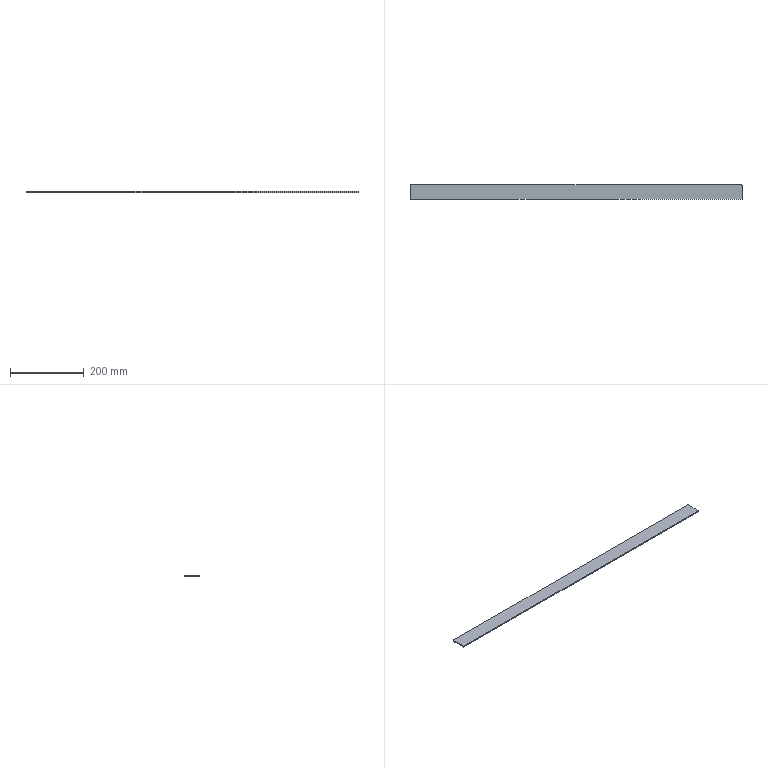Part | SolidWorks | features Extrusion 1, Fillet 1 | 1 solid | 8 faces | box 900 x 40 x 3 mm | volume 107995 mm3 | plane 6 | cylinder 2 | commonest cylinder face diameters 4 x2
STEP:
#1=CARTESIAN_POINT('',(450.,-20.,0.));
#2=VERTEX_POINT('',#1);
#3=CARTESIAN_POINT('',(450.,18.,0.));
#4=VERTEX_POINT('',#3);
#5=CARTESIAN_POINT('',(450.,20.,0.));
#6=DIRECTION('',(0.,1.,0.));
#7=VECTOR('',#6,1000.);
#8=LINE('',#5,#7);
#9=EDGE_CURVE('',#2,#4,#8,.T.);
#10=ORIENTED_EDGE('',*,*,#9,.T.);
#11=CARTESIAN_POINT('',(450.,18.,3.));
#12=VERTEX_POINT('',#11);
#13=CARTESIAN_POINT('',(450.,18.,3.));
#14=DIRECTION('',(0.,0.,1.));
#15=VECTOR('',#14,1000.);
#16=LINE('',#13,#15);
#17=EDGE_CURVE('',#4,#12,#16,.T.);
#18=ORIENTED_EDGE('',*,*,#17,.T.);
#19=CARTESIAN_POINT('',(450.,-20.,3.));
#20=VERTEX_POINT('',#19);
#21=CARTESIAN_POINT('',(450.,20.,3.));
#22=DIRECTION('',(0.,1.,0.));
#23=VECTOR('',#22,1000.);
#24=LINE('',#21,#23);
#25=EDGE_CURVE('',#20,#12,#24,.T.);
#26=ORIENTED_EDGE('',*,*,#25,.F.);
#27=CARTESIAN_POINT('',(450.,-20.,3.));
#28=DIRECTION('',(0.,0.,-1.));
#29=VECTOR('',#28,1000.);
#30=LINE('',#27,#29);
#31=EDGE_CURVE('',#20,#2,#30,.T.);
#32=ORIENTED_EDGE('',*,*,#31,.T.);
#33=EDGE_LOOP('',(#10,#18,#26,#32));
#34=FACE_OUTER_BOUND('',#33,.T.);
#35=CARTESIAN_POINT('',(450.,20.,3.));
#36=DIRECTION('',(-1.,0.,0.));
#37=DIRECTION('',(0.,0.,1.));
#38=AXIS2_PLACEMENT_3D('',#35,#36,#37);
#39=PLANE('',#38);
#40=ADVANCED_FACE('',(#34),#39,.F.);
#41=CARTESIAN_POINT('',(448.,20.,0.));
#42=VERTEX_POINT('',#41);
#43=CARTESIAN_POINT('',(-448.,20.,0.));
#44=VERTEX_POINT('',#43);
#45=CARTESIAN_POINT('',(-450.,20.,0.));
#46=DIRECTION('',(-1.,0.,0.));
#47=VECTOR('',#46,1000.);
#48=LINE('',#45,#47);
#49=EDGE_CURVE('',#42,#44,#48,.T.);
#50=ORIENTED_EDGE('',*,*,#49,.T.);
#51=CARTESIAN_POINT('',(-448.,20.,3.));
#52=VERTEX_POINT('',#51);
#53=CARTESIAN_POINT('',(-448.,20.,3.));
#54=DIRECTION('',(0.,0.,1.));
#55=VECTOR('',#54,1000.);
#56=LINE('',#53,#55);
#57=EDGE_CURVE('',#44,#52,#56,.T.);
#58=ORIENTED_EDGE('',*,*,#57,.T.);
#59=CARTESIAN_POINT('',(448.,20.,3.));
#60=VERTEX_POINT('',#59);
#61=CARTESIAN_POINT('',(-450.,20.,3.));
#62=DIRECTION('',(-1.,0.,0.));
#63=VECTOR('',#62,1000.);
#64=LINE('',#61,#63);
#65=EDGE_CURVE('',#60,#52,#64,.T.);
#66=ORIENTED_EDGE('',*,*,#65,.F.);
#67=CARTESIAN_POINT('',(448.,20.,3.));
#68=DIRECTION('',(0.,0.,-1.));
#69=VECTOR('',#68,1000.);
#70=LINE('',#67,#69);
#71=EDGE_CURVE('',#60,#42,#70,.T.);
#72=ORIENTED_EDGE('',*,*,#71,.T.);
#73=EDGE_LOOP('',(#50,#58,#66,#72));
#74=FACE_OUTER_BOUND('',#73,.T.);
#75=CARTESIAN_POINT('',(-450.,20.,3.));
#76=DIRECTION('',(0.,-1.,0.));
#77=DIRECTION('',(0.,0.,-1.));
#78=AXIS2_PLACEMENT_3D('',#75,#76,#77);
#79=PLANE('',#78);
#80=ADVANCED_FACE('',(#74),#79,.F.);
#81=CARTESIAN_POINT('',(-450.,18.,3.));
#82=VERTEX_POINT('',#81);
#83=CARTESIAN_POINT('',(-450.,-20.,3.));
#84=VERTEX_POINT('',#83);
#85=CARTESIAN_POINT('',(-450.,20.,3.));
#86=DIRECTION('',(0.,-1.,0.));
#87=VECTOR('',#86,1000.);
#88=LINE('',#85,#87);
#89=EDGE_CURVE('',#82,#84,#88,.T.);
#90=ORIENTED_EDGE('',*,*,#89,.F.);
#91=CARTESIAN_POINT('',(-450.,18.,0.));
#92=VERTEX_POINT('',#91);
#93=CARTESIAN_POINT('',(-450.,18.,3.));
#94=DIRECTION('',(0.,0.,-1.));
#95=VECTOR('',#94,1000.);
#96=LINE('',#93,#95);
#97=EDGE_CURVE('',#82,#92,#96,.T.);
#98=ORIENTED_EDGE('',*,*,#97,.T.);
#99=CARTESIAN_POINT('',(-450.,-20.,0.));
#100=VERTEX_POINT('',#99);
#101=CARTESIAN_POINT('',(-450.,20.,0.));
#102=DIRECTION('',(0.,-1.,0.));
#103=VECTOR('',#102,1000.);
#104=LINE('',#101,#103);
#105=EDGE_CURVE('',#92,#100,#104,.T.);
#106=ORIENTED_EDGE('',*,*,#105,.T.);
#107=CARTESIAN_POINT('',(-450.,-20.,3.));
#108=DIRECTION('',(0.,0.,-1.));
#109=VECTOR('',#108,1000.);
#110=LINE('',#107,#109);
#111=EDGE_CURVE('',#84,#100,#110,.T.);
#112=ORIENTED_EDGE('',*,*,#111,.F.);
#113=EDGE_LOOP('',(#90,#98,#106,#112));
#114=FACE_OUTER_BOUND('',#113,.T.);
#115=CARTESIAN_POINT('',(-450.,20.,3.));
#116=DIRECTION('',(1.,0.,0.));
#117=DIRECTION('',(0.,1.,0.));
#118=AXIS2_PLACEMENT_3D('',#115,#116,#117);
#119=PLANE('',#118);
#120=ADVANCED_FACE('',(#114),#119,.F.);
#121=CARTESIAN_POINT('',(-450.,-20.,0.));
#122=DIRECTION('',(1.,0.,0.));
#123=VECTOR('',#122,1000.);
#124=LINE('',#121,#123);
#125=EDGE_CURVE('',#100,#2,#124,.T.);
#126=ORIENTED_EDGE('',*,*,#125,.T.);
#127=ORIENTED_EDGE('',*,*,#31,.F.);
#128=CARTESIAN_POINT('',(-450.,-20.,3.));
#129=DIRECTION('',(1.,0.,0.));
#130=VECTOR('',#129,1000.);
#131=LINE('',#128,#130);
#132=EDGE_CURVE('',#84,#20,#131,.T.);
#133=ORIENTED_EDGE('',*,*,#132,.F.);
#134=ORIENTED_EDGE('',*,*,#111,.T.);
#135=EDGE_LOOP('',(#126,#127,#133,#134));
#136=FACE_OUTER_BOUND('',#135,.T.);
#137=CARTESIAN_POINT('',(-450.,-20.,3.));
#138=DIRECTION('',(0.,1.,0.));
#139=DIRECTION('',(0.,0.,1.));
#140=AXIS2_PLACEMENT_3D('',#137,#138,#139);
#141=PLANE('',#140);
#142=ADVANCED_FACE('',(#136),#141,.F.);
#143=ORIENTED_EDGE('',*,*,#65,.T.);
#144=CARTESIAN_POINT('',(-448.,18.,3.));
#145=DIRECTION('',(0.,0.,1.));
#146=DIRECTION('',(1.,0.,0.));
#147=AXIS2_PLACEMENT_3D('',#144,#145,#146);
#148=CIRCLE('',#147,2.);
#149=EDGE_CURVE('',#52,#82,#148,.T.);
#150=ORIENTED_EDGE('',*,*,#149,.T.);
#151=ORIENTED_EDGE('',*,*,#89,.T.);
#152=ORIENTED_EDGE('',*,*,#132,.T.);
#153=ORIENTED_EDGE('',*,*,#25,.T.);
#154=CARTESIAN_POINT('',(448.,18.,3.));
#155=DIRECTION('',(0.,0.,1.));
#156=DIRECTION('',(1.,0.,0.));
#157=AXIS2_PLACEMENT_3D('',#154,#155,#156);
#158=CIRCLE('',#157,2.);
#159=EDGE_CURVE('',#12,#60,#158,.T.);
#160=ORIENTED_EDGE('',*,*,#159,.T.);
#161=EDGE_LOOP('',(#143,#150,#151,#152,#153,#160));
#162=FACE_OUTER_BOUND('',#161,.T.);
#163=CARTESIAN_POINT('',(0.,0.,3.));
#164=DIRECTION('',(0.,0.,1.));
#165=DIRECTION('',(1.,0.,0.));
#166=AXIS2_PLACEMENT_3D('',#163,#164,#165);
#167=PLANE('',#166);
#168=ADVANCED_FACE('',(#162),#167,.T.);
#169=ORIENTED_EDGE('',*,*,#105,.F.);
#170=CARTESIAN_POINT('',(-448.,18.,0.));
#171=DIRECTION('',(0.,0.,-1.));
#172=DIRECTION('',(1.,0.,0.));
#173=AXIS2_PLACEMENT_3D('',#170,#171,#172);
#174=CIRCLE('',#173,2.);
#175=EDGE_CURVE('',#92,#44,#174,.T.);
#176=ORIENTED_EDGE('',*,*,#175,.T.);
#177=ORIENTED_EDGE('',*,*,#49,.F.);
#178=CARTESIAN_POINT('',(448.,18.,0.));
#179=DIRECTION('',(0.,0.,-1.));
#180=DIRECTION('',(1.,0.,0.));
#181=AXIS2_PLACEMENT_3D('',#178,#179,#180);
#182=CIRCLE('',#181,2.);
#183=EDGE_CURVE('',#42,#4,#182,.T.);
#184=ORIENTED_EDGE('',*,*,#183,.T.);
#185=ORIENTED_EDGE('',*,*,#9,.F.);
#186=ORIENTED_EDGE('',*,*,#125,.F.);
#187=EDGE_LOOP('',(#169,#176,#177,#184,#185,#186));
#188=FACE_OUTER_BOUND('',#187,.T.);
#189=CARTESIAN_POINT('',(0.,0.,0.));
#190=DIRECTION('',(0.,0.,1.));
#191=DIRECTION('',(1.,0.,0.));
#192=AXIS2_PLACEMENT_3D('',#189,#190,#191);
#193=PLANE('',#192);
#194=ADVANCED_FACE('',(#188),#193,.F.);
#195=ORIENTED_EDGE('',*,*,#149,.F.);
#196=ORIENTED_EDGE('',*,*,#57,.F.);
#197=ORIENTED_EDGE('',*,*,#175,.F.);
#198=ORIENTED_EDGE('',*,*,#97,.F.);
#199=EDGE_LOOP('',(#195,#196,#197,#198));
#200=FACE_OUTER_BOUND('',#199,.T.);
#201=CARTESIAN_POINT('',(-448.,18.,3.));
#202=DIRECTION('',(0.,0.,-1.));
#203=DIRECTION('',(-1.,0.,0.));
#204=AXIS2_PLACEMENT_3D('',#201,#202,#203);
#205=CYLINDRICAL_SURFACE('',#204,2.);
#206=ADVANCED_FACE('',(#200),#205,.T.);
#207=ORIENTED_EDGE('',*,*,#159,.F.);
#208=ORIENTED_EDGE('',*,*,#17,.F.);
#209=ORIENTED_EDGE('',*,*,#183,.F.);
#210=ORIENTED_EDGE('',*,*,#71,.F.);
#211=EDGE_LOOP('',(#207,#208,#209,#210));
#212=FACE_OUTER_BOUND('',#211,.T.);
#213=CARTESIAN_POINT('',(448.,18.,3.));
#214=DIRECTION('',(0.,0.,-1.));
#215=DIRECTION('',(-1.,0.,0.));
#216=AXIS2_PLACEMENT_3D('',#213,#214,#215);
#217=CYLINDRICAL_SURFACE('',#216,2.);
#218=ADVANCED_FACE('',(#212),#217,.T.);
#219=CLOSED_SHELL('',(#40,#80,#120,#142,#168,#194,#206,#218));
#220=MANIFOLD_SOLID_BREP('',#219);
#221=CARTESIAN_POINT('',(0.,0.,0.));
#222=DIRECTION('',(0.,0.,1.));
#223=DIRECTION('',(1.,0.,0.));
#224=AXIS2_PLACEMENT_3D('',#221,#222,#223);
#225=(LENGTH_UNIT()NAMED_UNIT(*)SI_UNIT(.MILLI.,.METRE.));
#226=UNCERTAINTY_MEASURE_WITH_UNIT(LENGTH_MEASURE(0.00001),#225,'','');
#227=(NAMED_UNIT(*)PLANE_ANGLE_UNIT()SI_UNIT($,.RADIAN.));
#228=(NAMED_UNIT(*)SI_UNIT($,.STERADIAN.)SOLID_ANGLE_UNIT());
#229=(GEOMETRIC_REPRESENTATION_CONTEXT(3)GLOBAL_UNCERTAINTY_ASSIGNED_CONTEXT((#226))GLOBAL_UNIT_ASSIGNED_CONTEXT((#225,#227,#228))REPRESENTATION_CONTEXT('',''));
#230=ADVANCED_BREP_SHAPE_REPRESENTATION('',(#220,#224),#229);